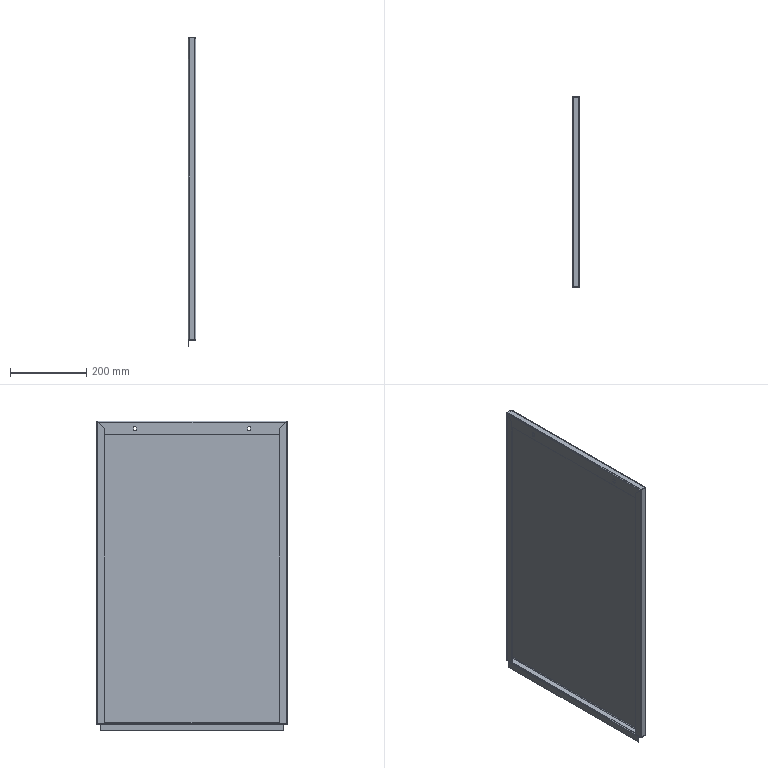Part | NX | features solid 2 | 1 solid | 104 faces | box 20 x 500 x 814 mm | volume 734939 mm3 | plane 70 | cylinder 26 | spline 8 | commonest cylinder face diameters 3 x8 6 x8 7 x6 20 x2 23 x2